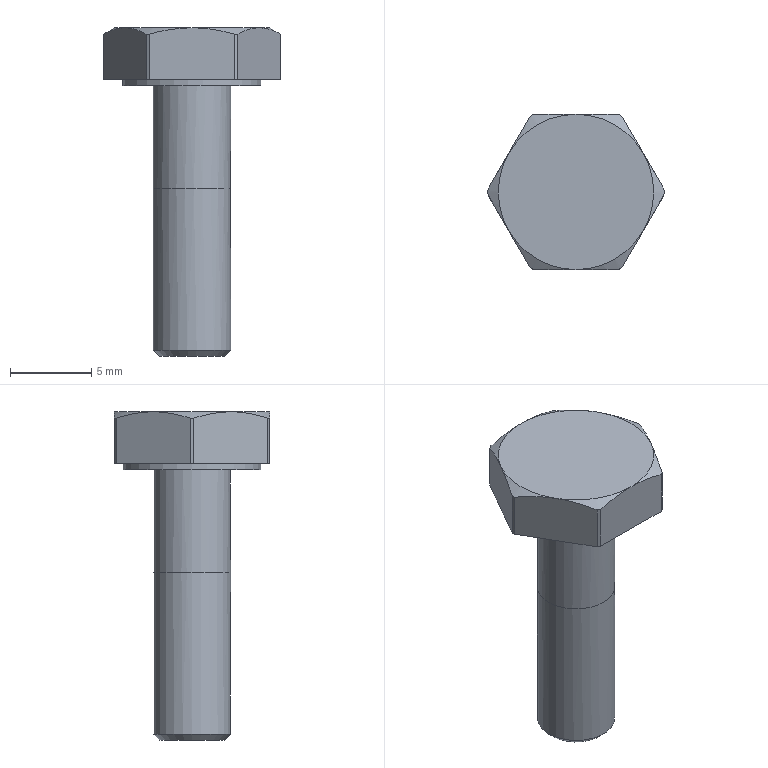Part | NX | features solid 2 | 1 solid | 26 faces | box 10.922 x 9.576 x 20.25 mm | volume 570.047 mm3 | plane 10 | cylinder 9 | cone 7 | commonest cylinder face diameters 10.922 x6 4.763 x2 8.509 x1
STEP:
#1=CARTESIAN_POINT('',(-2.381,0.,-3.581));
#2=VERTEX_POINT('',#1);
#3=CARTESIAN_POINT('',(0.,0.,-3.581));
#4=DIRECTION('',(0.,0.,-1.));
#5=DIRECTION('',(-1.,0.,0.));
#6=AXIS2_PLACEMENT_3D('',#3,#4,#5);
#7=CIRCLE('',#6,2.381);
#8=EDGE_CURVE('',#2,#2,#7,.T.);
#9=ORIENTED_EDGE('',*,*,#8,.T.);
#10=EDGE_LOOP('',(#9));
#11=FACE_BOUND('',#10,.T.);
#12=CARTESIAN_POINT('',(-2.381,0.,-9.931));
#13=VERTEX_POINT('',#12);
#14=CARTESIAN_POINT('',(-1.866,1.866,-9.931));
#15=CARTESIAN_POINT('',(-2.639,0.,-9.931));
#16=CARTESIAN_POINT('',(-1.866,-1.866,-9.931));
#17=CARTESIAN_POINT('',(0.,-2.639,-9.931));
#18=CARTESIAN_POINT('',(1.866,-1.866,-9.931));
#19=CARTESIAN_POINT('',(2.639,0.,-9.931));
#20=CARTESIAN_POINT('',(1.866,1.866,-9.931));
#21=CARTESIAN_POINT('',(0.,2.639,-9.931));
#22=CARTESIAN_POINT('',(-1.866,1.866,-9.931));
#23=CARTESIAN_POINT('',(-2.639,0.,-9.931));
#24=CARTESIAN_POINT('',(-1.866,-1.866,-9.931));
#25=B_SPLINE_CURVE_WITH_KNOTS('',3,(#14,#15,#16,#17,#18,#19,#20,#21,#22,#23,#24),.UNSPECIFIED.,.T.,.F.,(1,1,1,1,1,1,1,1,1,1,1,1,1,1,1),(-0.375,-0.25,-0.125,0.,0.125,0.25,0.375,0.5,0.625,0.75,0.875,1.,1.125,1.25,1.375),.UNSPECIFIED.);
#26=EDGE_CURVE('',#13,#13,#25,.T.);
#27=ORIENTED_EDGE('',*,*,#26,.T.);
#28=EDGE_LOOP('',(#27));
#29=FACE_BOUND('',#28,.T.);
#30=CARTESIAN_POINT('',(0.,0.,0.));
#31=DIRECTION('',(0.,0.,-1.));
#32=DIRECTION('',(-1.,0.,0.));
#33=AXIS2_PLACEMENT_3D('',#30,#31,#32);
#34=CYLINDRICAL_SURFACE('',#33,2.381);
#35=ADVANCED_FACE('',(#11,#29),#34,.T.);
#36=CARTESIAN_POINT('',(2.627,4.788,-3.175));
#37=VERTEX_POINT('',#36);
#38=CARTESIAN_POINT('',(2.833,4.669,-3.175));
#39=VERTEX_POINT('',#38);
#40=CARTESIAN_POINT('',(0.,0.,-3.175));
#41=DIRECTION('',(0.,0.,-1.));
#42=DIRECTION('',(-1.,0.,0.));
#43=AXIS2_PLACEMENT_3D('',#40,#41,#42);
#44=CIRCLE('',#43,5.461);
#45=EDGE_CURVE('',#37,#39,#44,.T.);
#46=ORIENTED_EDGE('',*,*,#45,.F.);
#47=CARTESIAN_POINT('',(2.627,4.788,-0.3886));
#48=VERTEX_POINT('',#47);
#49=CARTESIAN_POINT('',(2.627,4.788,0.));
#50=DIRECTION('',(0.,0.,-1.));
#51=VECTOR('',#50,1000.);
#52=LINE('',#49,#51);
#53=EDGE_CURVE('',#37,#48,#52,.F.);
#54=ORIENTED_EDGE('',*,*,#53,.T.);
#55=CARTESIAN_POINT('',(2.833,4.669,-0.3886));
#56=VERTEX_POINT('',#55);
#57=CARTESIAN_POINT('',(0.,0.,-0.3886));
#58=DIRECTION('',(0.,0.,-1.));
#59=DIRECTION('',(-1.,0.,0.));
#60=AXIS2_PLACEMENT_3D('',#57,#58,#59);
#61=CIRCLE('',#60,5.461);
#62=EDGE_CURVE('',#48,#56,#61,.T.);
#63=ORIENTED_EDGE('',*,*,#62,.T.);
#64=CARTESIAN_POINT('',(2.833,4.669,0.));
#65=DIRECTION('',(0.,0.,-1.));
#66=VECTOR('',#65,1000.);
#67=LINE('',#64,#66);
#68=EDGE_CURVE('',#56,#39,#67,.T.);
#69=ORIENTED_EDGE('',*,*,#68,.T.);
#70=EDGE_LOOP('',(#46,#54,#63,#69));
#71=FACE_BOUND('',#70,.T.);
#72=CARTESIAN_POINT('',(0.,0.,0.));
#73=DIRECTION('',(0.,0.,-1.));
#74=DIRECTION('',(-1.,0.,0.));
#75=AXIS2_PLACEMENT_3D('',#72,#73,#74);
#76=CYLINDRICAL_SURFACE('',#75,5.461);
#77=ADVANCED_FACE('',(#71),#76,.T.);
#78=CARTESIAN_POINT('',(-2.833,4.669,-0.3886));
#79=VERTEX_POINT('',#78);
#80=CARTESIAN_POINT('',(-2.627,4.788,-0.3886));
#81=VERTEX_POINT('',#80);
#82=CARTESIAN_POINT('',(0.,0.,-0.3886));
#83=DIRECTION('',(0.,0.,-1.));
#84=DIRECTION('',(-1.,0.,0.));
#85=AXIS2_PLACEMENT_3D('',#82,#83,#84);
#86=CIRCLE('',#85,5.461);
#87=EDGE_CURVE('',#79,#81,#86,.T.);
#88=ORIENTED_EDGE('',*,*,#87,.T.);
#89=CARTESIAN_POINT('',(-2.627,4.788,-3.175));
#90=VERTEX_POINT('',#89);
#91=CARTESIAN_POINT('',(-2.627,4.788,0.));
#92=DIRECTION('',(0.,0.,-1.));
#93=VECTOR('',#92,1000.);
#94=LINE('',#91,#93);
#95=EDGE_CURVE('',#81,#90,#94,.T.);
#96=ORIENTED_EDGE('',*,*,#95,.T.);
#97=CARTESIAN_POINT('',(-2.833,4.669,-3.175));
#98=VERTEX_POINT('',#97);
#99=CARTESIAN_POINT('',(0.,0.,-3.175));
#100=DIRECTION('',(0.,0.,-1.));
#101=DIRECTION('',(-1.,0.,0.));
#102=AXIS2_PLACEMENT_3D('',#99,#100,#101);
#103=CIRCLE('',#102,5.461);
#104=EDGE_CURVE('',#98,#90,#103,.T.);
#105=ORIENTED_EDGE('',*,*,#104,.F.);
#106=CARTESIAN_POINT('',(-2.833,4.669,0.));
#107=DIRECTION('',(0.,0.,-1.));
#108=VECTOR('',#107,1000.);
#109=LINE('',#106,#108);
#110=EDGE_CURVE('',#98,#79,#109,.F.);
#111=ORIENTED_EDGE('',*,*,#110,.T.);
#112=EDGE_LOOP('',(#88,#96,#105,#111));
#113=FACE_BOUND('',#112,.T.);
#114=CARTESIAN_POINT('',(0.,0.,0.));
#115=DIRECTION('',(0.,0.,-1.));
#116=DIRECTION('',(-1.,0.,0.));
#117=AXIS2_PLACEMENT_3D('',#114,#115,#116);
#118=CYLINDRICAL_SURFACE('',#117,5.461);
#119=ADVANCED_FACE('',(#113),#118,.T.);
#120=CARTESIAN_POINT('',(-5.46,-0.1193,-0.3886));
#121=VERTEX_POINT('',#120);
#122=CARTESIAN_POINT('',(-5.46,0.1193,-0.3886));
#123=VERTEX_POINT('',#122);
#124=CARTESIAN_POINT('',(0.,0.,-0.3886));
#125=DIRECTION('',(0.,0.,-1.));
#126=DIRECTION('',(-1.,0.,0.));
#127=AXIS2_PLACEMENT_3D('',#124,#125,#126);
#128=CIRCLE('',#127,5.461);
#129=EDGE_CURVE('',#121,#123,#128,.T.);
#130=ORIENTED_EDGE('',*,*,#129,.T.);
#131=CARTESIAN_POINT('',(-5.46,0.1193,-3.175));
#132=VERTEX_POINT('',#131);
#133=CARTESIAN_POINT('',(-5.46,0.1193,0.));
#134=DIRECTION('',(0.,0.,-1.));
#135=VECTOR('',#134,1000.);
#136=LINE('',#133,#135);
#137=EDGE_CURVE('',#123,#132,#136,.T.);
#138=ORIENTED_EDGE('',*,*,#137,.T.);
#139=CARTESIAN_POINT('',(-5.46,-0.1193,-3.175));
#140=VERTEX_POINT('',#139);
#141=CARTESIAN_POINT('',(0.,0.,-3.175));
#142=DIRECTION('',(0.,0.,-1.));
#143=DIRECTION('',(-1.,0.,0.));
#144=AXIS2_PLACEMENT_3D('',#141,#142,#143);
#145=CIRCLE('',#144,5.461);
#146=EDGE_CURVE('',#140,#132,#145,.T.);
#147=ORIENTED_EDGE('',*,*,#146,.F.);
#148=CARTESIAN_POINT('',(-5.46,-0.1193,0.));
#149=DIRECTION('',(0.,0.,-1.));
#150=VECTOR('',#149,1000.);
#151=LINE('',#148,#150);
#152=EDGE_CURVE('',#140,#121,#151,.F.);
#153=ORIENTED_EDGE('',*,*,#152,.T.);
#154=EDGE_LOOP('',(#130,#138,#147,#153));
#155=FACE_BOUND('',#154,.T.);
#156=CARTESIAN_POINT('',(0.,0.,0.));
#157=DIRECTION('',(0.,0.,-1.));
#158=DIRECTION('',(-1.,0.,0.));
#159=AXIS2_PLACEMENT_3D('',#156,#157,#158);
#160=CYLINDRICAL_SURFACE('',#159,5.461);
#161=ADVANCED_FACE('',(#155),#160,.T.);
#162=CARTESIAN_POINT('',(-2.627,-4.788,-0.3886));
#163=VERTEX_POINT('',#162);
#164=CARTESIAN_POINT('',(-2.833,-4.669,-0.3886));
#165=VERTEX_POINT('',#164);
#166=CARTESIAN_POINT('',(0.,0.,-0.3886));
#167=DIRECTION('',(0.,0.,-1.));
#168=DIRECTION('',(-1.,0.,0.));
#169=AXIS2_PLACEMENT_3D('',#166,#167,#168);
#170=CIRCLE('',#169,5.461);
#171=EDGE_CURVE('',#163,#165,#170,.T.);
#172=ORIENTED_EDGE('',*,*,#171,.T.);
#173=CARTESIAN_POINT('',(-2.833,-4.669,-3.175));
#174=VERTEX_POINT('',#173);
#175=CARTESIAN_POINT('',(-2.833,-4.669,0.));
#176=DIRECTION('',(0.,0.,-1.));
#177=VECTOR('',#176,1000.);
#178=LINE('',#175,#177);
#179=EDGE_CURVE('',#165,#174,#178,.T.);
#180=ORIENTED_EDGE('',*,*,#179,.T.);
#181=CARTESIAN_POINT('',(-2.627,-4.788,-3.175));
#182=VERTEX_POINT('',#181);
#183=CARTESIAN_POINT('',(0.,0.,-3.175));
#184=DIRECTION('',(0.,0.,-1.));
#185=DIRECTION('',(-1.,0.,0.));
#186=AXIS2_PLACEMENT_3D('',#183,#184,#185);
#187=CIRCLE('',#186,5.461);
#188=EDGE_CURVE('',#182,#174,#187,.T.);
#189=ORIENTED_EDGE('',*,*,#188,.F.);
#190=CARTESIAN_POINT('',(-2.627,-4.788,0.));
#191=DIRECTION('',(0.,0.,-1.));
#192=VECTOR('',#191,1000.);
#193=LINE('',#190,#192);
#194=EDGE_CURVE('',#182,#163,#193,.F.);
#195=ORIENTED_EDGE('',*,*,#194,.T.);
#196=EDGE_LOOP('',(#172,#180,#189,#195));
#197=FACE_BOUND('',#196,.T.);
#198=CARTESIAN_POINT('',(0.,0.,0.));
#199=DIRECTION('',(0.,0.,-1.));
#200=DIRECTION('',(-1.,0.,0.));
#201=AXIS2_PLACEMENT_3D('',#198,#199,#200);
#202=CYLINDRICAL_SURFACE('',#201,5.461);
#203=ADVANCED_FACE('',(#197),#202,.T.);
#204=CARTESIAN_POINT('',(2.833,-4.669,-0.3886));
#205=VERTEX_POINT('',#204);
#206=CARTESIAN_POINT('',(2.627,-4.788,-0.3886));
#207=VERTEX_POINT('',#206);
#208=CARTESIAN_POINT('',(0.,0.,-0.3886));
#209=DIRECTION('',(0.,0.,-1.));
#210=DIRECTION('',(-1.,0.,0.));
#211=AXIS2_PLACEMENT_3D('',#208,#209,#210);
#212=CIRCLE('',#211,5.461);
#213=EDGE_CURVE('',#205,#207,#212,.T.);
#214=ORIENTED_EDGE('',*,*,#213,.T.);
#215=CARTESIAN_POINT('',(2.627,-4.788,-3.175));
#216=VERTEX_POINT('',#215);
#217=CARTESIAN_POINT('',(2.627,-4.788,0.));
#218=DIRECTION('',(0.,0.,-1.));
#219=VECTOR('',#218,1000.);
#220=LINE('',#217,#219);
#221=EDGE_CURVE('',#207,#216,#220,.T.);
#222=ORIENTED_EDGE('',*,*,#221,.T.);
#223=CARTESIAN_POINT('',(2.833,-4.669,-3.175));
#224=VERTEX_POINT('',#223);
#225=CARTESIAN_POINT('',(0.,0.,-3.175));
#226=DIRECTION('',(0.,0.,-1.));
#227=DIRECTION('',(-1.,0.,0.));
#228=AXIS2_PLACEMENT_3D('',#225,#226,#227);
#229=CIRCLE('',#228,5.461);
#230=EDGE_CURVE('',#224,#216,#229,.T.);
#231=ORIENTED_EDGE('',*,*,#230,.F.);
#232=CARTESIAN_POINT('',(2.833,-4.669,0.));
#233=DIRECTION('',(0.,0.,-1.));
#234=VECTOR('',#233,1000.);
#235=LINE('',#232,#234);
#236=EDGE_CURVE('',#224,#205,#235,.F.);
#237=ORIENTED_EDGE('',*,*,#236,.T.);
#238=EDGE_LOOP('',(#214,#222,#231,#237));
#239=FACE_BOUND('',#238,.T.);
#240=CARTESIAN_POINT('',(0.,0.,0.));
#241=DIRECTION('',(0.,0.,-1.));
#242=DIRECTION('',(-1.,0.,0.));
#243=AXIS2_PLACEMENT_3D('',#240,#241,#242);
#244=CYLINDRICAL_SURFACE('',#243,5.461);
#245=ADVANCED_FACE('',(#239),#244,.T.);
#246=ORIENTED_EDGE('',*,*,#62,.F.);
#247=CARTESIAN_POINT('',(0.,4.788,0.));
#248=VERTEX_POINT('',#247);
#249=CARTESIAN_POINT('',(0.,4.788,0.));
#250=CARTESIAN_POINT('',(0.8868,4.788,0.));
#251=CARTESIAN_POINT('',(1.776,4.788,-0.1525));
#252=CARTESIAN_POINT('',(2.627,4.788,-0.3886));
#253=B_SPLINE_CURVE_WITH_KNOTS('',3,(#249,#250,#251,#252),.UNSPECIFIED.,.F.,.F.,(4,4),(0.007722,0.01038),.UNSPECIFIED.);
#254=EDGE_CURVE('',#48,#248,#253,.F.);
#255=ORIENTED_EDGE('',*,*,#254,.T.);
#256=CARTESIAN_POINT('',(4.146,2.394,0.));
#257=VERTEX_POINT('',#256);
#258=CARTESIAN_POINT('',(0.,0.,0.));
#259=DIRECTION('',(0.,0.,-1.));
#260=DIRECTION('',(-1.,0.,0.));
#261=AXIS2_PLACEMENT_3D('',#258,#259,#260);
#262=CIRCLE('',#261,4.788);
#263=EDGE_CURVE('',#248,#257,#262,.T.);
#264=ORIENTED_EDGE('',*,*,#263,.T.);
#265=CARTESIAN_POINT('',(4.146,2.394,0.));
#266=CARTESIAN_POINT('',(3.703,3.163,0.));
#267=CARTESIAN_POINT('',(3.262,3.925,-0.1503));
#268=CARTESIAN_POINT('',(2.833,4.669,-0.3886));
#269=B_SPLINE_CURVE_WITH_KNOTS('',3,(#265,#266,#267,#268),.UNSPECIFIED.,.F.,.F.,(4,4),(0.002655,0.005296),.UNSPECIFIED.);
#270=EDGE_CURVE('',#257,#56,#269,.T.);
#271=ORIENTED_EDGE('',*,*,#270,.T.);
#272=EDGE_LOOP('',(#246,#255,#264,#271));
#273=FACE_BOUND('',#272,.T.);
#274=CARTESIAN_POINT('',(0.,0.,-0.3886));
#275=DIRECTION('',(0.,0.,-1.));
#276=DIRECTION('',(-1.,0.,0.));
#277=AXIS2_PLACEMENT_3D('',#274,#275,#276);
#278=CONICAL_SURFACE('',#277,5.461,1.047);
#279=ADVANCED_FACE('',(#273),#278,.T.);
#280=CARTESIAN_POINT('',(-4.146,2.394,0.));
#281=VERTEX_POINT('',#280);
#282=CARTESIAN_POINT('',(0.,0.,0.));
#283=DIRECTION('',(0.,0.,-1.));
#284=DIRECTION('',(-1.,0.,0.));
#285=AXIS2_PLACEMENT_3D('',#282,#283,#284);
#286=CIRCLE('',#285,4.788);
#287=EDGE_CURVE('',#281,#248,#286,.T.);
#288=ORIENTED_EDGE('',*,*,#287,.T.);
#289=CARTESIAN_POINT('',(-2.627,4.788,-0.3886));
#290=CARTESIAN_POINT('',(-1.77,4.788,-0.1508));
#291=CARTESIAN_POINT('',(-0.8866,4.788,0.));
#292=CARTESIAN_POINT('',(0.,4.788,0.));
#293=B_SPLINE_CURVE_WITH_KNOTS('',3,(#289,#290,#291,#292),.UNSPECIFIED.,.F.,.F.,(4,4),(0.005068,0.007722),.UNSPECIFIED.);
#294=EDGE_CURVE('',#248,#81,#293,.F.);
#295=ORIENTED_EDGE('',*,*,#294,.T.);
#296=ORIENTED_EDGE('',*,*,#87,.F.);
#297=CARTESIAN_POINT('',(-2.833,4.669,-0.3886));
#298=CARTESIAN_POINT('',(-3.264,3.923,-0.1495));
#299=CARTESIAN_POINT('',(-3.7,3.167,0.));
#300=CARTESIAN_POINT('',(-4.146,2.394,0.));
#301=B_SPLINE_CURVE_WITH_KNOTS('',3,(#297,#298,#299,#300),.UNSPECIFIED.,.F.,.F.,(4,4),(0.00000074,0.002655),.UNSPECIFIED.);
#302=EDGE_CURVE('',#79,#281,#301,.T.);
#303=ORIENTED_EDGE('',*,*,#302,.T.);
#304=EDGE_LOOP('',(#288,#295,#296,#303));
#305=FACE_BOUND('',#304,.T.);
#306=CARTESIAN_POINT('',(0.,0.,-0.3886));
#307=DIRECTION('',(0.,0.,-1.));
#308=DIRECTION('',(-1.,0.,0.));
#309=AXIS2_PLACEMENT_3D('',#306,#307,#308);
#310=CONICAL_SURFACE('',#309,5.461,1.047);
#311=ADVANCED_FACE('',(#305),#310,.T.);
#312=CARTESIAN_POINT('',(-4.146,-2.394,0.));
#313=VERTEX_POINT('',#312);
#314=CARTESIAN_POINT('',(0.,0.,0.));
#315=DIRECTION('',(0.,0.,-1.));
#316=DIRECTION('',(-1.,0.,0.));
#317=AXIS2_PLACEMENT_3D('',#314,#315,#316);
#318=CIRCLE('',#317,4.788);
#319=EDGE_CURVE('',#313,#281,#318,.T.);
#320=ORIENTED_EDGE('',*,*,#319,.T.);
#321=CARTESIAN_POINT('',(-4.146,2.394,0.));
#322=CARTESIAN_POINT('',(-4.59,1.625,0.));
#323=CARTESIAN_POINT('',(-5.031,0.8625,-0.1503));
#324=CARTESIAN_POINT('',(-5.46,0.1193,-0.3886));
#325=B_SPLINE_CURVE_WITH_KNOTS('',3,(#321,#322,#323,#324),.UNSPECIFIED.,.F.,.F.,(4,4),(0.002655,0.005296),.UNSPECIFIED.);
#326=EDGE_CURVE('',#281,#123,#325,.T.);
#327=ORIENTED_EDGE('',*,*,#326,.T.);
#328=ORIENTED_EDGE('',*,*,#129,.F.);
#329=CARTESIAN_POINT('',(-5.46,-0.1193,-0.3886));
#330=CARTESIAN_POINT('',(-5.029,-0.8651,-0.1495));
#331=CARTESIAN_POINT('',(-4.593,-1.621,0.));
#332=CARTESIAN_POINT('',(-4.146,-2.394,0.));
#333=B_SPLINE_CURVE_WITH_KNOTS('',3,(#329,#330,#331,#332),.UNSPECIFIED.,.F.,.F.,(4,4),(0.00000074,0.002655),.UNSPECIFIED.);
#334=EDGE_CURVE('',#121,#313,#333,.T.);
#335=ORIENTED_EDGE('',*,*,#334,.T.);
#336=EDGE_LOOP('',(#320,#327,#328,#335));
#337=FACE_BOUND('',#336,.T.);
#338=CARTESIAN_POINT('',(0.,0.,-0.3886));
#339=DIRECTION('',(0.,0.,-1.));
#340=DIRECTION('',(-1.,0.,0.));
#341=AXIS2_PLACEMENT_3D('',#338,#339,#340);
#342=CONICAL_SURFACE('',#341,5.461,1.047);
#343=ADVANCED_FACE('',(#337),#342,.T.);
#344=CARTESIAN_POINT('',(0.,-4.788,0.));
#345=VERTEX_POINT('',#344);
#346=CARTESIAN_POINT('',(0.,0.,0.));
#347=DIRECTION('',(0.,0.,-1.));
#348=DIRECTION('',(-1.,0.,0.));
#349=AXIS2_PLACEMENT_3D('',#346,#347,#348);
#350=CIRCLE('',#349,4.788);
#351=EDGE_CURVE('',#345,#313,#350,.T.);
#352=ORIENTED_EDGE('',*,*,#351,.T.);
#353=CARTESIAN_POINT('',(-4.146,-2.394,0.));
#354=CARTESIAN_POINT('',(-3.703,-3.163,0.));
#355=CARTESIAN_POINT('',(-3.262,-3.925,-0.1503));
#356=CARTESIAN_POINT('',(-2.833,-4.669,-0.3886));
#357=B_SPLINE_CURVE_WITH_KNOTS('',3,(#353,#354,#355,#356),.UNSPECIFIED.,.F.,.F.,(4,4),(0.002655,0.005296),.UNSPECIFIED.);
#358=EDGE_CURVE('',#313,#165,#357,.T.);
#359=ORIENTED_EDGE('',*,*,#358,.T.);
#360=ORIENTED_EDGE('',*,*,#171,.F.);
#361=CARTESIAN_POINT('',(-2.627,-4.788,-0.3886));
#362=CARTESIAN_POINT('',(-1.77,-4.788,-0.1508));
#363=CARTESIAN_POINT('',(-0.8866,-4.788,0.));
#364=CARTESIAN_POINT('',(0.,-4.788,0.));
#365=B_SPLINE_CURVE_WITH_KNOTS('',3,(#361,#362,#363,#364),.UNSPECIFIED.,.F.,.F.,(4,4),(0.005068,0.007722),.UNSPECIFIED.);
#366=EDGE_CURVE('',#163,#345,#365,.T.);
#367=ORIENTED_EDGE('',*,*,#366,.T.);
#368=EDGE_LOOP('',(#352,#359,#360,#367));
#369=FACE_BOUND('',#368,.T.);
#370=CARTESIAN_POINT('',(0.,0.,-0.3886));
#371=DIRECTION('',(0.,0.,-1.));
#372=DIRECTION('',(-1.,0.,0.));
#373=AXIS2_PLACEMENT_3D('',#370,#371,#372);
#374=CONICAL_SURFACE('',#373,5.461,1.047);
#375=ADVANCED_FACE('',(#369),#374,.T.);
#376=CARTESIAN_POINT('',(4.146,-2.394,0.));
#377=VERTEX_POINT('',#376);
#378=CARTESIAN_POINT('',(0.,0.,0.));
#379=DIRECTION('',(0.,0.,-1.));
#380=DIRECTION('',(-1.,0.,0.));
#381=AXIS2_PLACEMENT_3D('',#378,#379,#380);
#382=CIRCLE('',#381,4.788);
#383=EDGE_CURVE('',#377,#345,#382,.T.);
#384=ORIENTED_EDGE('',*,*,#383,.T.);
#385=CARTESIAN_POINT('',(0.,-4.788,0.));
#386=CARTESIAN_POINT('',(0.8868,-4.788,0.));
#387=CARTESIAN_POINT('',(1.776,-4.788,-0.1525));
#388=CARTESIAN_POINT('',(2.627,-4.788,-0.3886));
#389=B_SPLINE_CURVE_WITH_KNOTS('',3,(#385,#386,#387,#388),.UNSPECIFIED.,.F.,.F.,(4,4),(0.007722,0.01038),.UNSPECIFIED.);
#390=EDGE_CURVE('',#345,#207,#389,.T.);
#391=ORIENTED_EDGE('',*,*,#390,.T.);
#392=ORIENTED_EDGE('',*,*,#213,.F.);
#393=CARTESIAN_POINT('',(2.833,-4.669,-0.3886));
#394=CARTESIAN_POINT('',(3.264,-3.923,-0.1495));
#395=CARTESIAN_POINT('',(3.7,-3.167,0.));
#396=CARTESIAN_POINT('',(4.146,-2.394,0.));
#397=B_SPLINE_CURVE_WITH_KNOTS('',3,(#393,#394,#395,#396),.UNSPECIFIED.,.F.,.F.,(4,4),(0.00000074,0.002655),.UNSPECIFIED.);
#398=EDGE_CURVE('',#205,#377,#397,.T.);
#399=ORIENTED_EDGE('',*,*,#398,.T.);
#400=EDGE_LOOP('',(#384,#391,#392,#399));
#401=FACE_BOUND('',#400,.T.);
#402=CARTESIAN_POINT('',(0.,0.,-0.3886));
#403=DIRECTION('',(0.,0.,-1.));
#404=DIRECTION('',(-1.,0.,0.));
#405=AXIS2_PLACEMENT_3D('',#402,#403,#404);
#406=CONICAL_SURFACE('',#405,5.461,1.047);
#407=ADVANCED_FACE('',(#401),#406,.T.);
#408=ORIENTED_EDGE('',*,*,#104,.T.);
#409=CARTESIAN_POINT('',(4.255,4.788,-3.175));
#410=DIRECTION('',(1.,0.,0.));
#411=VECTOR('',#410,1000.);
#412=LINE('',#409,#411);
#413=EDGE_CURVE('',#90,#37,#412,.T.);
#414=ORIENTED_EDGE('',*,*,#413,.T.);
#415=ORIENTED_EDGE('',*,*,#45,.T.);
#416=CARTESIAN_POINT('',(5.46,0.1193,-3.175));
#417=VERTEX_POINT('',#416);
#418=CARTESIAN_POINT('',(5.21,0.5517,-3.175));
#419=DIRECTION('',(0.5,-0.866,0.));
#420=VECTOR('',#419,1000.);
#421=LINE('',#418,#420);
#422=EDGE_CURVE('',#39,#417,#421,.T.);
#423=ORIENTED_EDGE('',*,*,#422,.T.);
#424=CARTESIAN_POINT('',(5.46,-0.1193,-3.175));
#425=VERTEX_POINT('',#424);
#426=CARTESIAN_POINT('',(0.,0.,-3.175));
#427=DIRECTION('',(0.,0.,-1.));
#428=DIRECTION('',(-1.,0.,0.));
#429=AXIS2_PLACEMENT_3D('',#426,#427,#428);
#430=CIRCLE('',#429,5.461);
#431=EDGE_CURVE('',#417,#425,#430,.T.);
#432=ORIENTED_EDGE('',*,*,#431,.T.);
#433=CARTESIAN_POINT('',(5.21,-0.5517,-3.175));
#434=DIRECTION('',(-0.5,-0.866,0.));
#435=VECTOR('',#434,1000.);
#436=LINE('',#433,#435);
#437=EDGE_CURVE('',#425,#224,#436,.T.);
#438=ORIENTED_EDGE('',*,*,#437,.T.);
#439=ORIENTED_EDGE('',*,*,#230,.T.);
#440=CARTESIAN_POINT('',(4.255,-4.788,-3.175));
#441=DIRECTION('',(-1.,0.,0.));
#442=VECTOR('',#441,1000.);
#443=LINE('',#440,#442);
#444=EDGE_CURVE('',#216,#182,#443,.T.);
#445=ORIENTED_EDGE('',*,*,#444,.T.);
#446=ORIENTED_EDGE('',*,*,#188,.T.);
#447=CARTESIAN_POINT('',(-3.083,-4.236,-3.175));
#448=DIRECTION('',(-0.5,0.866,0.));
#449=VECTOR('',#448,1000.);
#450=LINE('',#447,#449);
#451=EDGE_CURVE('',#174,#140,#450,.T.);
#452=ORIENTED_EDGE('',*,*,#451,.T.);
#453=ORIENTED_EDGE('',*,*,#146,.T.);
#454=CARTESIAN_POINT('',(-3.083,4.236,-3.175));
#455=DIRECTION('',(0.5,0.866,0.));
#456=VECTOR('',#455,1000.);
#457=LINE('',#454,#456);
#458=EDGE_CURVE('',#132,#98,#457,.T.);
#459=ORIENTED_EDGE('',*,*,#458,.T.);
#460=EDGE_LOOP('',(#408,#414,#415,#423,#432,#438,#439,#445,#446,#452,#453,#459));
#461=FACE_BOUND('',#460,.T.);
#462=CARTESIAN_POINT('',(-4.255,0.,-3.175));
#463=VERTEX_POINT('',#462);
#464=CARTESIAN_POINT('',(0.,0.,-3.175));
#465=DIRECTION('',(0.,0.,-1.));
#466=DIRECTION('',(-1.,0.,0.));
#467=AXIS2_PLACEMENT_3D('',#464,#465,#466);
#468=CIRCLE('',#467,4.255);
#469=EDGE_CURVE('',#463,#463,#468,.T.);
#470=ORIENTED_EDGE('',*,*,#469,.F.);
#471=EDGE_LOOP('',(#470));
#472=FACE_BOUND('',#471,.T.);
#473=CARTESIAN_POINT('',(4.255,0.,-3.175));
#474=DIRECTION('',(0.,0.,-1.));
#475=DIRECTION('',(-1.,0.,0.));
#476=AXIS2_PLACEMENT_3D('',#473,#474,#475);
#477=PLANE('',#476);
#478=ADVANCED_FACE('',(#461,#472),#477,.T.);
#479=CARTESIAN_POINT('',(5.46,0.1193,-0.3886));
#480=VERTEX_POINT('',#479);
#481=CARTESIAN_POINT('',(5.46,-0.1193,-0.3886));
#482=VERTEX_POINT('',#481);
#483=CARTESIAN_POINT('',(0.,0.,-0.3886));
#484=DIRECTION('',(0.,0.,-1.));
#485=DIRECTION('',(-1.,0.,0.));
#486=AXIS2_PLACEMENT_3D('',#483,#484,#485);
#487=CIRCLE('',#486,5.461);
#488=EDGE_CURVE('',#480,#482,#487,.T.);
#489=ORIENTED_EDGE('',*,*,#488,.T.);
#490=CARTESIAN_POINT('',(5.46,-0.1193,0.));
#491=DIRECTION('',(0.,0.,-1.));
#492=VECTOR('',#491,1000.);
#493=LINE('',#490,#492);
#494=EDGE_CURVE('',#482,#425,#493,.T.);
#495=ORIENTED_EDGE('',*,*,#494,.T.);
#496=ORIENTED_EDGE('',*,*,#431,.F.);
#497=CARTESIAN_POINT('',(5.46,0.1193,0.));
#498=DIRECTION('',(0.,0.,-1.));
#499=VECTOR('',#498,1000.);
#500=LINE('',#497,#499);
#501=EDGE_CURVE('',#417,#480,#500,.F.);
#502=ORIENTED_EDGE('',*,*,#501,.T.);
#503=EDGE_LOOP('',(#489,#495,#496,#502));
#504=FACE_BOUND('',#503,.T.);
#505=CARTESIAN_POINT('',(0.,0.,0.));
#506=DIRECTION('',(0.,0.,-1.));
#507=DIRECTION('',(-1.,0.,0.));
#508=AXIS2_PLACEMENT_3D('',#505,#506,#507);
#509=CYLINDRICAL_SURFACE('',#508,5.461);
#510=ADVANCED_FACE('',(#504),#509,.T.);
#511=CARTESIAN_POINT('',(0.,0.,0.));
#512=DIRECTION('',(0.,0.,-1.));
#513=DIRECTION('',(-1.,0.,0.));
#514=AXIS2_PLACEMENT_3D('',#511,#512,#513);
#515=CIRCLE('',#514,4.788);
#516=EDGE_CURVE('',#257,#377,#515,.T.);
#517=ORIENTED_EDGE('',*,*,#516,.T.);
#518=CARTESIAN_POINT('',(4.146,-2.394,0.));
#519=CARTESIAN_POINT('',(4.59,-1.625,0.));
#520=CARTESIAN_POINT('',(5.031,-0.8625,-0.1503));
#521=CARTESIAN_POINT('',(5.46,-0.1193,-0.3886));
#522=B_SPLINE_CURVE_WITH_KNOTS('',3,(#518,#519,#520,#521),.UNSPECIFIED.,.F.,.F.,(4,4),(0.002655,0.005296),.UNSPECIFIED.);
#523=EDGE_CURVE('',#377,#482,#522,.T.);
#524=ORIENTED_EDGE('',*,*,#523,.T.);
#525=ORIENTED_EDGE('',*,*,#488,.F.);
#526=CARTESIAN_POINT('',(5.46,0.1193,-0.3886));
#527=CARTESIAN_POINT('',(5.029,0.8651,-0.1495));
#528=CARTESIAN_POINT('',(4.593,1.621,0.));
#529=CARTESIAN_POINT('',(4.146,2.394,0.));
#530=B_SPLINE_CURVE_WITH_KNOTS('',3,(#526,#527,#528,#529),.UNSPECIFIED.,.F.,.F.,(4,4),(0.00000074,0.002655),.UNSPECIFIED.);
#531=EDGE_CURVE('',#480,#257,#530,.T.);
#532=ORIENTED_EDGE('',*,*,#531,.T.);
#533=EDGE_LOOP('',(#517,#524,#525,#532));
#534=FACE_BOUND('',#533,.T.);
#535=CARTESIAN_POINT('',(0.,0.,-0.3886));
#536=DIRECTION('',(0.,0.,-1.));
#537=DIRECTION('',(-1.,0.,0.));
#538=AXIS2_PLACEMENT_3D('',#535,#536,#537);
#539=CONICAL_SURFACE('',#538,5.461,1.047);
#540=ADVANCED_FACE('',(#534),#539,.T.);
#541=ORIENTED_EDGE('',*,*,#287,.F.);
#542=ORIENTED_EDGE('',*,*,#319,.F.);
#543=ORIENTED_EDGE('',*,*,#351,.F.);
#544=ORIENTED_EDGE('',*,*,#383,.F.);
#545=ORIENTED_EDGE('',*,*,#516,.F.);
#546=ORIENTED_EDGE('',*,*,#263,.F.);
#547=EDGE_LOOP('',(#541,#542,#543,#544,#545,#546));
#548=FACE_BOUND('',#547,.T.);
#549=CARTESIAN_POINT('',(4.788,0.,0.));
#550=DIRECTION('',(0.,0.,1.));
#551=DIRECTION('',(1.,0.,0.));
#552=AXIS2_PLACEMENT_3D('',#549,#550,#551);
#553=PLANE('',#552);
#554=ADVANCED_FACE('',(#548),#553,.T.);
#555=CARTESIAN_POINT('',(-2.,0.,-20.25));
#556=VERTEX_POINT('',#555);
#557=CARTESIAN_POINT('',(0.,0.,-20.25));
#558=DIRECTION('',(0.,0.,-1.));
#559=DIRECTION('',(-1.,0.,0.));
#560=AXIS2_PLACEMENT_3D('',#557,#558,#559);
#561=CIRCLE('',#560,2.);
#562=EDGE_CURVE('',#556,#556,#561,.T.);
#563=ORIENTED_EDGE('',*,*,#562,.T.);
#564=EDGE_LOOP('',(#563));
#565=FACE_BOUND('',#564,.T.);
#566=CARTESIAN_POINT('',(0.,0.,-20.25));
#567=DIRECTION('',(0.,0.,-1.));
#568=DIRECTION('',(-1.,0.,0.));
#569=AXIS2_PLACEMENT_3D('',#566,#567,#568);
#570=PLANE('',#569);
#571=ADVANCED_FACE('',(#565),#570,.T.);
#572=CARTESIAN_POINT('',(-2.381,0.,-19.869));
#573=VERTEX_POINT('',#572);
#574=CARTESIAN_POINT('',(0.,0.,-19.869));
#575=DIRECTION('',(0.,0.,-1.));
#576=DIRECTION('',(-1.,0.,0.));
#577=AXIS2_PLACEMENT_3D('',#574,#575,#576);
#578=CIRCLE('',#577,2.381);
#579=EDGE_CURVE('',#573,#573,#578,.T.);
#580=ORIENTED_EDGE('',*,*,#579,.T.);
#581=EDGE_LOOP('',(#580));
#582=FACE_BOUND('',#581,.T.);
#583=ORIENTED_EDGE('',*,*,#562,.F.);
#584=EDGE_LOOP('',(#583));
#585=FACE_BOUND('',#584,.T.);
#586=CARTESIAN_POINT('',(0.,0.,-20.25));
#587=DIRECTION('',(0.,0.,1.));
#588=DIRECTION('',(1.,0.,0.));
#589=AXIS2_PLACEMENT_3D('',#586,#587,#588);
#590=CONICAL_SURFACE('',#589,2.,0.7854);
#591=ADVANCED_FACE('',(#582,#585),#590,.T.);
#592=ORIENTED_EDGE('',*,*,#26,.F.);
#593=EDGE_LOOP('',(#592));
#594=FACE_BOUND('',#593,.T.);
#595=ORIENTED_EDGE('',*,*,#579,.F.);
#596=EDGE_LOOP('',(#595));
#597=FACE_BOUND('',#596,.T.);
#598=CARTESIAN_POINT('',(0.,0.,0.));
#599=DIRECTION('',(0.,0.,-1.));
#600=DIRECTION('',(-1.,0.,0.));
#601=AXIS2_PLACEMENT_3D('',#598,#599,#600);
#602=CYLINDRICAL_SURFACE('',#601,2.381);
#603=ADVANCED_FACE('',(#594,#597),#602,.T.);
#604=CARTESIAN_POINT('',(-4.255,0.,-3.581));
#605=VERTEX_POINT('',#604);
#606=CARTESIAN_POINT('',(0.,0.,-3.581));
#607=DIRECTION('',(0.,0.,-1.));
#608=DIRECTION('',(-1.,0.,0.));
#609=AXIS2_PLACEMENT_3D('',#606,#607,#608);
#610=CIRCLE('',#609,4.255);
#611=EDGE_CURVE('',#605,#605,#610,.T.);
#612=ORIENTED_EDGE('',*,*,#611,.T.);
#613=EDGE_LOOP('',(#612));
#614=FACE_BOUND('',#613,.T.);
#615=ORIENTED_EDGE('',*,*,#8,.F.);
#616=EDGE_LOOP('',(#615));
#617=FACE_BOUND('',#616,.T.);
#618=CARTESIAN_POINT('',(2.381,0.,-3.581));
#619=DIRECTION('',(0.,0.,-1.));
#620=DIRECTION('',(-1.,0.,0.));
#621=AXIS2_PLACEMENT_3D('',#618,#619,#620);
#622=PLANE('',#621);
#623=ADVANCED_FACE('',(#614,#617),#622,.T.);
#624=ORIENTED_EDGE('',*,*,#469,.T.);
#625=EDGE_LOOP('',(#624));
#626=FACE_BOUND('',#625,.T.);
#627=ORIENTED_EDGE('',*,*,#611,.F.);
#628=EDGE_LOOP('',(#627));
#629=FACE_BOUND('',#628,.T.);
#630=CARTESIAN_POINT('',(0.,0.,0.));
#631=DIRECTION('',(0.,0.,-1.));
#632=DIRECTION('',(-1.,0.,0.));
#633=AXIS2_PLACEMENT_3D('',#630,#631,#632);
#634=CYLINDRICAL_SURFACE('',#633,4.255);
#635=ADVANCED_FACE('',(#626,#629),#634,.T.);
#636=ORIENTED_EDGE('',*,*,#422,.F.);
#637=ORIENTED_EDGE('',*,*,#68,.F.);
#638=ORIENTED_EDGE('',*,*,#270,.F.);
#639=ORIENTED_EDGE('',*,*,#531,.F.);
#640=ORIENTED_EDGE('',*,*,#501,.F.);
#641=EDGE_LOOP('',(#636,#637,#638,#639,#640));
#642=FACE_BOUND('',#641,.T.);
#643=CARTESIAN_POINT('',(5.529,0.,-22.275));
#644=DIRECTION('',(0.866,0.5,0.));
#645=DIRECTION('',(-0.5,0.866,0.));
#646=AXIS2_PLACEMENT_3D('',#643,#644,#645);
#647=PLANE('',#646);
#648=ADVANCED_FACE('',(#642),#647,.T.);
#649=ORIENTED_EDGE('',*,*,#437,.F.);
#650=ORIENTED_EDGE('',*,*,#494,.F.);
#651=ORIENTED_EDGE('',*,*,#523,.F.);
#652=ORIENTED_EDGE('',*,*,#398,.F.);
#653=ORIENTED_EDGE('',*,*,#236,.F.);
#654=EDGE_LOOP('',(#649,#650,#651,#652,#653));
#655=FACE_BOUND('',#654,.T.);
#656=CARTESIAN_POINT('',(2.764,-4.788,-22.275));
#657=DIRECTION('',(0.866,-0.5,0.));
#658=DIRECTION('',(0.5,0.866,0.));
#659=AXIS2_PLACEMENT_3D('',#656,#657,#658);
#660=PLANE('',#659);
#661=ADVANCED_FACE('',(#655),#660,.T.);
#662=ORIENTED_EDGE('',*,*,#444,.F.);
#663=ORIENTED_EDGE('',*,*,#221,.F.);
#664=ORIENTED_EDGE('',*,*,#390,.F.);
#665=ORIENTED_EDGE('',*,*,#366,.F.);
#666=ORIENTED_EDGE('',*,*,#194,.F.);
#667=EDGE_LOOP('',(#662,#663,#664,#665,#666));
#668=FACE_BOUND('',#667,.T.);
#669=CARTESIAN_POINT('',(-2.764,-4.788,-22.275));
#670=DIRECTION('',(0.,-1.,0.));
#671=DIRECTION('',(0.,0.,-1.));
#672=AXIS2_PLACEMENT_3D('',#669,#670,#671);
#673=PLANE('',#672);
#674=ADVANCED_FACE('',(#668),#673,.T.);
#675=ORIENTED_EDGE('',*,*,#451,.F.);
#676=ORIENTED_EDGE('',*,*,#179,.F.);
#677=ORIENTED_EDGE('',*,*,#358,.F.);
#678=ORIENTED_EDGE('',*,*,#334,.F.);
#679=ORIENTED_EDGE('',*,*,#152,.F.);
#680=EDGE_LOOP('',(#675,#676,#677,#678,#679));
#681=FACE_BOUND('',#680,.T.);
#682=CARTESIAN_POINT('',(-5.529,0.,-22.275));
#683=DIRECTION('',(-0.866,-0.5,0.));
#684=DIRECTION('',(0.5,-0.866,0.));
#685=AXIS2_PLACEMENT_3D('',#682,#683,#684);
#686=PLANE('',#685);
#687=ADVANCED_FACE('',(#681),#686,.T.);
#688=ORIENTED_EDGE('',*,*,#458,.F.);
#689=ORIENTED_EDGE('',*,*,#137,.F.);
#690=ORIENTED_EDGE('',*,*,#326,.F.);
#691=ORIENTED_EDGE('',*,*,#302,.F.);
#692=ORIENTED_EDGE('',*,*,#110,.F.);
#693=EDGE_LOOP('',(#688,#689,#690,#691,#692));
#694=FACE_BOUND('',#693,.T.);
#695=CARTESIAN_POINT('',(-2.764,4.788,-22.275));
#696=DIRECTION('',(-0.866,0.5,0.));
#697=DIRECTION('',(-0.5,-0.866,0.));
#698=AXIS2_PLACEMENT_3D('',#695,#696,#697);
#699=PLANE('',#698);
#700=ADVANCED_FACE('',(#694),#699,.T.);
#701=ORIENTED_EDGE('',*,*,#413,.F.);
#702=ORIENTED_EDGE('',*,*,#95,.F.);
#703=ORIENTED_EDGE('',*,*,#294,.F.);
#704=ORIENTED_EDGE('',*,*,#254,.F.);
#705=ORIENTED_EDGE('',*,*,#53,.F.);
#706=EDGE_LOOP('',(#701,#702,#703,#704,#705));
#707=FACE_BOUND('',#706,.T.);
#708=CARTESIAN_POINT('',(2.764,4.788,-22.275));
#709=DIRECTION('',(0.,1.,0.));
#710=DIRECTION('',(0.,0.,1.));
#711=AXIS2_PLACEMENT_3D('',#708,#709,#710);
#712=PLANE('',#711);
#713=ADVANCED_FACE('',(#707),#712,.T.);
#714=CLOSED_SHELL('',(#35,#77,#119,#161,#203,#245,#279,#311,#343,#375,#407,#478,#510,#540,#554,#571,#591,#603,#623,#635,#648,#661,#674,#687,#700,#713));
#715=MANIFOLD_SOLID_BREP('',#714);
#716=(LENGTH_UNIT()NAMED_UNIT(*)SI_UNIT(.MILLI.,.METRE.));
#717=UNCERTAINTY_MEASURE_WITH_UNIT(LENGTH_MEASURE(0.0508),#716,'','');
#718=(NAMED_UNIT(*)PLANE_ANGLE_UNIT()SI_UNIT($,.RADIAN.));
#719=(NAMED_UNIT(*)SI_UNIT($,.STERADIAN.)SOLID_ANGLE_UNIT());
#720=(GEOMETRIC_REPRESENTATION_CONTEXT(3)GLOBAL_UNCERTAINTY_ASSIGNED_CONTEXT((#717))GLOBAL_UNIT_ASSIGNED_CONTEXT((#716,#718,#719))REPRESENTATION_CONTEXT('',''));
#721=ADVANCED_BREP_SHAPE_REPRESENTATION('',(#715),#720);